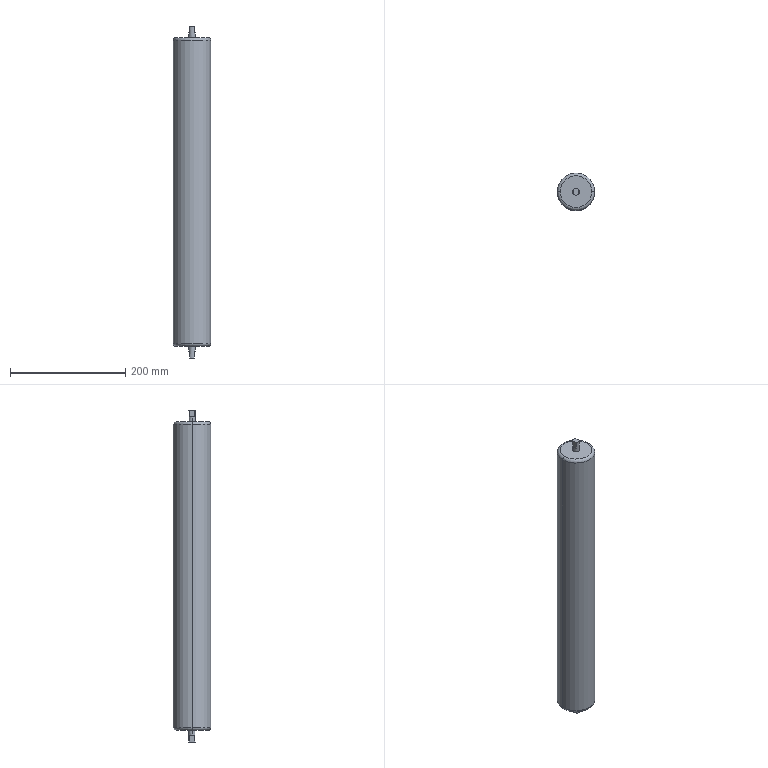Part | SolidWorks | features ICE 2, Extrusion 1, Fillet 1, MirrorPattern 1 | 1 solid | 22 faces | box 65 x 65 x 575 mm | volume 1777108 mm3 | plane 12 | cylinder 6 | torus 4 | commonest cylinder face diameters 12 x4 65 x2
STEP:
#1=CARTESIAN_POINT('',(-27.5,0.,-267.5));
#2=VERTEX_POINT('',#1);
#3=CARTESIAN_POINT('',(27.5,0.,-267.5));
#4=VERTEX_POINT('',#3);
#5=CARTESIAN_POINT('',(0.,0.,-267.5));
#6=DIRECTION('',(0.,0.,-1.));
#7=DIRECTION('',(1.,0.,0.));
#8=AXIS2_PLACEMENT_3D('',#5,#6,#7);
#9=CIRCLE('',#8,27.5);
#10=EDGE_CURVE('',#2,#4,#9,.T.);
#11=ORIENTED_EDGE('',*,*,#10,.F.);
#12=CARTESIAN_POINT('',(-32.5,0.,-262.5));
#13=VERTEX_POINT('',#12);
#14=CARTESIAN_POINT('',(-27.5,0.,-262.5));
#15=DIRECTION('',(0.,1.,0.));
#16=DIRECTION('',(-1.,0.,0.));
#17=AXIS2_PLACEMENT_3D('',#14,#15,#16);
#18=CIRCLE('',#17,5.);
#19=EDGE_CURVE('',#2,#13,#18,.T.);
#20=ORIENTED_EDGE('',*,*,#19,.T.);
#21=CARTESIAN_POINT('',(32.5,0.,-262.5));
#22=VERTEX_POINT('',#21);
#23=CARTESIAN_POINT('',(0.,0.,-262.5));
#24=DIRECTION('',(0.,0.,1.));
#25=DIRECTION('',(1.,0.,0.));
#26=AXIS2_PLACEMENT_3D('',#23,#24,#25);
#27=CIRCLE('',#26,32.5);
#28=EDGE_CURVE('',#22,#13,#27,.T.);
#29=ORIENTED_EDGE('',*,*,#28,.F.);
#30=CARTESIAN_POINT('',(27.5,0.,-262.5));
#31=DIRECTION('',(0.,-1.,0.));
#32=DIRECTION('',(0.,0.,-1.));
#33=AXIS2_PLACEMENT_3D('',#30,#31,#32);
#34=CIRCLE('',#33,5.);
#35=EDGE_CURVE('',#4,#22,#34,.T.);
#36=ORIENTED_EDGE('',*,*,#35,.F.);
#37=EDGE_LOOP('',(#11,#20,#29,#36));
#38=FACE_OUTER_BOUND('',#37,.T.);
#39=CARTESIAN_POINT('',(0.,0.,-262.5));
#40=DIRECTION('',(0.,0.,1.));
#41=DIRECTION('',(1.,0.,0.));
#42=AXIS2_PLACEMENT_3D('',#39,#40,#41);
#43=TOROIDAL_SURFACE('',#42,27.5,5.);
#44=ADVANCED_FACE('',(#38),#43,.T.);
#45=CARTESIAN_POINT('',(-32.5,0.,262.5));
#46=VERTEX_POINT('',#45);
#47=CARTESIAN_POINT('',(32.5,0.,262.5));
#48=VERTEX_POINT('',#47);
#49=CARTESIAN_POINT('',(0.,0.,262.5));
#50=DIRECTION('',(0.,0.,-1.));
#51=DIRECTION('',(1.,0.,0.));
#52=AXIS2_PLACEMENT_3D('',#49,#50,#51);
#53=CIRCLE('',#52,32.5);
#54=EDGE_CURVE('',#46,#48,#53,.T.);
#55=ORIENTED_EDGE('',*,*,#54,.F.);
#56=CARTESIAN_POINT('',(-27.5,0.,267.5));
#57=VERTEX_POINT('',#56);
#58=CARTESIAN_POINT('',(-27.5,0.,262.5));
#59=DIRECTION('',(0.,1.,0.));
#60=DIRECTION('',(-1.,0.,0.));
#61=AXIS2_PLACEMENT_3D('',#58,#59,#60);
#62=CIRCLE('',#61,5.);
#63=EDGE_CURVE('',#46,#57,#62,.T.);
#64=ORIENTED_EDGE('',*,*,#63,.T.);
#65=CARTESIAN_POINT('',(27.5,0.,267.5));
#66=VERTEX_POINT('',#65);
#67=CARTESIAN_POINT('',(0.,0.,267.5));
#68=DIRECTION('',(0.,0.,1.));
#69=DIRECTION('',(1.,0.,0.));
#70=AXIS2_PLACEMENT_3D('',#67,#68,#69);
#71=CIRCLE('',#70,27.5);
#72=EDGE_CURVE('',#66,#57,#71,.T.);
#73=ORIENTED_EDGE('',*,*,#72,.F.);
#74=CARTESIAN_POINT('',(27.5,0.,262.5));
#75=DIRECTION('',(0.,-1.,0.));
#76=DIRECTION('',(0.,0.,-1.));
#77=AXIS2_PLACEMENT_3D('',#74,#75,#76);
#78=CIRCLE('',#77,5.);
#79=EDGE_CURVE('',#48,#66,#78,.T.);
#80=ORIENTED_EDGE('',*,*,#79,.F.);
#81=EDGE_LOOP('',(#55,#64,#73,#80));
#82=FACE_OUTER_BOUND('',#81,.T.);
#83=CARTESIAN_POINT('',(0.,0.,262.5));
#84=DIRECTION('',(0.,0.,1.));
#85=DIRECTION('',(1.,0.,0.));
#86=AXIS2_PLACEMENT_3D('',#83,#84,#85);
#87=TOROIDAL_SURFACE('',#86,27.5,5.);
#88=ADVANCED_FACE('',(#82),#87,.T.);
#89=CARTESIAN_POINT('',(4.,4.472,275.5));
#90=VERTEX_POINT('',#89);
#91=CARTESIAN_POINT('',(6.,0.,275.5));
#92=VERTEX_POINT('',#91);
#93=CARTESIAN_POINT('',(0.,0.,275.5));
#94=DIRECTION('',(0.,0.,-1.));
#95=DIRECTION('',(1.,0.,0.));
#96=AXIS2_PLACEMENT_3D('',#93,#94,#95);
#97=CIRCLE('',#96,6.);
#98=EDGE_CURVE('',#90,#92,#97,.T.);
#99=ORIENTED_EDGE('',*,*,#98,.T.);
#100=CARTESIAN_POINT('',(6.,0.,267.5));
#101=VERTEX_POINT('',#100);
#102=CARTESIAN_POINT('',(6.,0.,287.5));
#103=DIRECTION('',(0.,0.,-1.));
#104=VECTOR('',#103,1000.);
#105=LINE('',#102,#104);
#106=EDGE_CURVE('',#92,#101,#105,.T.);
#107=ORIENTED_EDGE('',*,*,#106,.T.);
#108=CARTESIAN_POINT('',(-6.,0.,267.5));
#109=VERTEX_POINT('',#108);
#110=CARTESIAN_POINT('',(0.,0.,267.5));
#111=DIRECTION('',(0.,0.,1.));
#112=DIRECTION('',(1.,0.,0.));
#113=AXIS2_PLACEMENT_3D('',#110,#111,#112);
#114=CIRCLE('',#113,6.);
#115=EDGE_CURVE('',#101,#109,#114,.T.);
#116=ORIENTED_EDGE('',*,*,#115,.T.);
#117=CARTESIAN_POINT('',(-6.,0.,275.5));
#118=VERTEX_POINT('',#117);
#119=CARTESIAN_POINT('',(-6.,0.,287.5));
#120=DIRECTION('',(0.,0.,-1.));
#121=VECTOR('',#120,1000.);
#122=LINE('',#119,#121);
#123=EDGE_CURVE('',#118,#109,#122,.T.);
#124=ORIENTED_EDGE('',*,*,#123,.F.);
#125=CARTESIAN_POINT('',(-4.,4.472,275.5));
#126=VERTEX_POINT('',#125);
#127=CARTESIAN_POINT('',(0.,0.,275.5));
#128=DIRECTION('',(0.,0.,-1.));
#129=DIRECTION('',(1.,0.,0.));
#130=AXIS2_PLACEMENT_3D('',#127,#128,#129);
#131=CIRCLE('',#130,6.);
#132=EDGE_CURVE('',#118,#126,#131,.T.);
#133=ORIENTED_EDGE('',*,*,#132,.T.);
#134=CARTESIAN_POINT('',(-4.,4.472,287.5));
#135=VERTEX_POINT('',#134);
#136=CARTESIAN_POINT('',(-4.,4.472,287.5));
#137=DIRECTION('',(0.,0.,-1.));
#138=VECTOR('',#137,1000.);
#139=LINE('',#136,#138);
#140=EDGE_CURVE('',#135,#126,#139,.T.);
#141=ORIENTED_EDGE('',*,*,#140,.F.);
#142=CARTESIAN_POINT('',(4.,4.472,287.5));
#143=VERTEX_POINT('',#142);
#144=CARTESIAN_POINT('',(0.,0.,287.5));
#145=DIRECTION('',(0.,0.,-1.));
#146=DIRECTION('',(-1.,0.,0.));
#147=AXIS2_PLACEMENT_3D('',#144,#145,#146);
#148=CIRCLE('',#147,6.);
#149=EDGE_CURVE('',#135,#143,#148,.T.);
#150=ORIENTED_EDGE('',*,*,#149,.T.);
#151=CARTESIAN_POINT('',(4.,4.472,287.5));
#152=DIRECTION('',(0.,0.,1.));
#153=VECTOR('',#152,1000.);
#154=LINE('',#151,#153);
#155=EDGE_CURVE('',#90,#143,#154,.T.);
#156=ORIENTED_EDGE('',*,*,#155,.F.);
#157=EDGE_LOOP('',(#99,#107,#116,#124,#133,#141,#150,#156));
#158=FACE_OUTER_BOUND('',#157,.T.);
#159=CARTESIAN_POINT('',(0.,0.,287.5));
#160=DIRECTION('',(0.,0.,-1.));
#161=DIRECTION('',(-1.,0.,0.));
#162=AXIS2_PLACEMENT_3D('',#159,#160,#161);
#163=CYLINDRICAL_SURFACE('',#162,6.);
#164=ADVANCED_FACE('',(#158),#163,.T.);
#165=ORIENTED_EDGE('',*,*,#54,.T.);
#166=CARTESIAN_POINT('',(32.5,0.,267.5));
#167=DIRECTION('',(0.,0.,-1.));
#168=VECTOR('',#167,1000.);
#169=LINE('',#166,#168);
#170=EDGE_CURVE('',#48,#22,#169,.T.);
#171=ORIENTED_EDGE('',*,*,#170,.T.);
#172=ORIENTED_EDGE('',*,*,#28,.T.);
#173=CARTESIAN_POINT('',(-32.5,0.,267.5));
#174=DIRECTION('',(0.,0.,-1.));
#175=VECTOR('',#174,1000.);
#176=LINE('',#173,#175);
#177=EDGE_CURVE('',#46,#13,#176,.T.);
#178=ORIENTED_EDGE('',*,*,#177,.F.);
#179=EDGE_LOOP('',(#165,#171,#172,#178));
#180=FACE_OUTER_BOUND('',#179,.T.);
#181=CARTESIAN_POINT('',(0.,0.,267.5));
#182=DIRECTION('',(0.,0.,-1.));
#183=DIRECTION('',(-1.,0.,0.));
#184=AXIS2_PLACEMENT_3D('',#181,#182,#183);
#185=CYLINDRICAL_SURFACE('',#184,32.5);
#186=ADVANCED_FACE('',(#180),#185,.T.);
#187=CARTESIAN_POINT('',(-6.,0.,-275.5));
#188=VERTEX_POINT('',#187);
#189=CARTESIAN_POINT('',(-4.,4.472,-275.5));
#190=VERTEX_POINT('',#189);
#191=CARTESIAN_POINT('',(0.,0.,-275.5));
#192=DIRECTION('',(0.,0.,-1.));
#193=DIRECTION('',(-1.,0.,0.));
#194=AXIS2_PLACEMENT_3D('',#191,#192,#193);
#195=CIRCLE('',#194,6.);
#196=EDGE_CURVE('',#188,#190,#195,.T.);
#197=ORIENTED_EDGE('',*,*,#196,.F.);
#198=CARTESIAN_POINT('',(-6.,0.,-267.5));
#199=VERTEX_POINT('',#198);
#200=CARTESIAN_POINT('',(-6.,0.,-287.5));
#201=DIRECTION('',(0.,0.,1.));
#202=VECTOR('',#201,1000.);
#203=LINE('',#200,#202);
#204=EDGE_CURVE('',#188,#199,#203,.T.);
#205=ORIENTED_EDGE('',*,*,#204,.T.);
#206=CARTESIAN_POINT('',(6.,0.,-267.5));
#207=VERTEX_POINT('',#206);
#208=CARTESIAN_POINT('',(0.,0.,-267.5));
#209=DIRECTION('',(0.,0.,-1.));
#210=DIRECTION('',(1.,0.,0.));
#211=AXIS2_PLACEMENT_3D('',#208,#209,#210);
#212=CIRCLE('',#211,6.);
#213=EDGE_CURVE('',#199,#207,#212,.T.);
#214=ORIENTED_EDGE('',*,*,#213,.T.);
#215=CARTESIAN_POINT('',(6.,0.,-275.5));
#216=VERTEX_POINT('',#215);
#217=CARTESIAN_POINT('',(6.,0.,-287.5));
#218=DIRECTION('',(0.,0.,1.));
#219=VECTOR('',#218,1000.);
#220=LINE('',#217,#219);
#221=EDGE_CURVE('',#216,#207,#220,.T.);
#222=ORIENTED_EDGE('',*,*,#221,.F.);
#223=CARTESIAN_POINT('',(4.,4.472,-275.5));
#224=VERTEX_POINT('',#223);
#225=CARTESIAN_POINT('',(0.,0.,-275.5));
#226=DIRECTION('',(0.,0.,-1.));
#227=DIRECTION('',(-1.,0.,0.));
#228=AXIS2_PLACEMENT_3D('',#225,#226,#227);
#229=CIRCLE('',#228,6.);
#230=EDGE_CURVE('',#224,#216,#229,.T.);
#231=ORIENTED_EDGE('',*,*,#230,.F.);
#232=CARTESIAN_POINT('',(4.,4.472,-287.5));
#233=VERTEX_POINT('',#232);
#234=CARTESIAN_POINT('',(4.,4.472,-287.5));
#235=DIRECTION('',(0.,0.,1.));
#236=VECTOR('',#235,1000.);
#237=LINE('',#234,#236);
#238=EDGE_CURVE('',#233,#224,#237,.T.);
#239=ORIENTED_EDGE('',*,*,#238,.F.);
#240=CARTESIAN_POINT('',(-4.,4.472,-287.5));
#241=VERTEX_POINT('',#240);
#242=CARTESIAN_POINT('',(0.,0.,-287.5));
#243=DIRECTION('',(0.,0.,-1.));
#244=DIRECTION('',(-1.,0.,0.));
#245=AXIS2_PLACEMENT_3D('',#242,#243,#244);
#246=CIRCLE('',#245,6.);
#247=EDGE_CURVE('',#241,#233,#246,.T.);
#248=ORIENTED_EDGE('',*,*,#247,.F.);
#249=CARTESIAN_POINT('',(-4.,4.472,-287.5));
#250=DIRECTION('',(0.,0.,-1.));
#251=VECTOR('',#250,1000.);
#252=LINE('',#249,#251);
#253=EDGE_CURVE('',#190,#241,#252,.T.);
#254=ORIENTED_EDGE('',*,*,#253,.F.);
#255=EDGE_LOOP('',(#197,#205,#214,#222,#231,#239,#248,#254));
#256=FACE_OUTER_BOUND('',#255,.T.);
#257=CARTESIAN_POINT('',(0.,0.,-287.5));
#258=DIRECTION('',(0.,0.,1.));
#259=DIRECTION('',(1.,0.,0.));
#260=AXIS2_PLACEMENT_3D('',#257,#258,#259);
#261=CYLINDRICAL_SURFACE('',#260,6.);
#262=ADVANCED_FACE('',(#256),#261,.T.);
#263=ORIENTED_EDGE('',*,*,#204,.F.);
#264=CARTESIAN_POINT('',(-4.,-4.472,-275.5));
#265=VERTEX_POINT('',#264);
#266=CARTESIAN_POINT('',(0.,0.,-275.5));
#267=DIRECTION('',(0.,0.,-1.));
#268=DIRECTION('',(-1.,0.,0.));
#269=AXIS2_PLACEMENT_3D('',#266,#267,#268);
#270=CIRCLE('',#269,6.);
#271=EDGE_CURVE('',#265,#188,#270,.T.);
#272=ORIENTED_EDGE('',*,*,#271,.F.);
#273=CARTESIAN_POINT('',(-4.,-4.472,-287.5));
#274=VERTEX_POINT('',#273);
#275=CARTESIAN_POINT('',(-4.,-4.472,-287.5));
#276=DIRECTION('',(0.,0.,1.));
#277=VECTOR('',#276,1000.);
#278=LINE('',#275,#277);
#279=EDGE_CURVE('',#274,#265,#278,.T.);
#280=ORIENTED_EDGE('',*,*,#279,.F.);
#281=CARTESIAN_POINT('',(4.,-4.472,-287.5));
#282=VERTEX_POINT('',#281);
#283=CARTESIAN_POINT('',(0.,0.,-287.5));
#284=DIRECTION('',(0.,0.,-1.));
#285=DIRECTION('',(-1.,0.,0.));
#286=AXIS2_PLACEMENT_3D('',#283,#284,#285);
#287=CIRCLE('',#286,6.);
#288=EDGE_CURVE('',#282,#274,#287,.T.);
#289=ORIENTED_EDGE('',*,*,#288,.F.);
#290=CARTESIAN_POINT('',(4.,-4.472,-275.5));
#291=VERTEX_POINT('',#290);
#292=CARTESIAN_POINT('',(4.,-4.472,-287.5));
#293=DIRECTION('',(0.,0.,-1.));
#294=VECTOR('',#293,1000.);
#295=LINE('',#292,#294);
#296=EDGE_CURVE('',#291,#282,#295,.T.);
#297=ORIENTED_EDGE('',*,*,#296,.F.);
#298=CARTESIAN_POINT('',(0.,0.,-275.5));
#299=DIRECTION('',(0.,0.,-1.));
#300=DIRECTION('',(-1.,0.,0.));
#301=AXIS2_PLACEMENT_3D('',#298,#299,#300);
#302=CIRCLE('',#301,6.);
#303=EDGE_CURVE('',#216,#291,#302,.T.);
#304=ORIENTED_EDGE('',*,*,#303,.F.);
#305=ORIENTED_EDGE('',*,*,#221,.T.);
#306=CARTESIAN_POINT('',(0.,0.,-267.5));
#307=DIRECTION('',(0.,0.,-1.));
#308=DIRECTION('',(1.,0.,0.));
#309=AXIS2_PLACEMENT_3D('',#306,#307,#308);
#310=CIRCLE('',#309,6.);
#311=EDGE_CURVE('',#207,#199,#310,.T.);
#312=ORIENTED_EDGE('',*,*,#311,.T.);
#313=EDGE_LOOP('',(#263,#272,#280,#289,#297,#304,#305,#312));
#314=FACE_OUTER_BOUND('',#313,.T.);
#315=CARTESIAN_POINT('',(0.,0.,-287.5));
#316=DIRECTION('',(0.,0.,1.));
#317=DIRECTION('',(1.,0.,0.));
#318=AXIS2_PLACEMENT_3D('',#315,#316,#317);
#319=CYLINDRICAL_SURFACE('',#318,6.);
#320=ADVANCED_FACE('',(#314),#319,.T.);
#321=ORIENTED_EDGE('',*,*,#288,.T.);
#322=CARTESIAN_POINT('',(-4.,0.,-287.5));
#323=DIRECTION('',(0.,1.,0.));
#324=VECTOR('',#323,1000.);
#325=LINE('',#322,#324);
#326=EDGE_CURVE('',#274,#241,#325,.T.);
#327=ORIENTED_EDGE('',*,*,#326,.T.);
#328=ORIENTED_EDGE('',*,*,#247,.T.);
#329=CARTESIAN_POINT('',(4.,0.,-287.5));
#330=DIRECTION('',(0.,-1.,0.));
#331=VECTOR('',#330,1000.);
#332=LINE('',#329,#331);
#333=EDGE_CURVE('',#233,#282,#332,.T.);
#334=ORIENTED_EDGE('',*,*,#333,.T.);
#335=EDGE_LOOP('',(#321,#327,#328,#334));
#336=FACE_OUTER_BOUND('',#335,.T.);
#337=CARTESIAN_POINT('',(0.,0.,-287.5));
#338=DIRECTION('',(0.,0.,-1.));
#339=DIRECTION('',(-1.,0.,0.));
#340=AXIS2_PLACEMENT_3D('',#337,#338,#339);
#341=PLANE('',#340);
#342=ADVANCED_FACE('',(#336),#341,.T.);
#343=CARTESIAN_POINT('',(0.,0.,-267.5));
#344=DIRECTION('',(0.,0.,-1.));
#345=DIRECTION('',(1.,0.,0.));
#346=AXIS2_PLACEMENT_3D('',#343,#344,#345);
#347=CIRCLE('',#346,27.5);
#348=EDGE_CURVE('',#4,#2,#347,.T.);
#349=ORIENTED_EDGE('',*,*,#348,.T.);
#350=ORIENTED_EDGE('',*,*,#10,.T.);
#351=EDGE_LOOP('',(#349,#350));
#352=FACE_OUTER_BOUND('',#351,.T.);
#353=ORIENTED_EDGE('',*,*,#311,.F.);
#354=ORIENTED_EDGE('',*,*,#213,.F.);
#355=EDGE_LOOP('',(#353,#354));
#356=FACE_BOUND('',#355,.T.);
#357=CARTESIAN_POINT('',(0.,0.,-267.5));
#358=DIRECTION('',(0.,0.,1.));
#359=DIRECTION('',(1.,0.,0.));
#360=AXIS2_PLACEMENT_3D('',#357,#358,#359);
#361=PLANE('',#360);
#362=ADVANCED_FACE('',(#352,#356),#361,.F.);
#363=ORIENTED_EDGE('',*,*,#170,.F.);
#364=CARTESIAN_POINT('',(0.,0.,262.5));
#365=DIRECTION('',(0.,0.,-1.));
#366=DIRECTION('',(1.,0.,0.));
#367=AXIS2_PLACEMENT_3D('',#364,#365,#366);
#368=CIRCLE('',#367,32.5);
#369=EDGE_CURVE('',#48,#46,#368,.T.);
#370=ORIENTED_EDGE('',*,*,#369,.T.);
#371=ORIENTED_EDGE('',*,*,#177,.T.);
#372=CARTESIAN_POINT('',(0.,0.,-262.5));
#373=DIRECTION('',(0.,0.,1.));
#374=DIRECTION('',(1.,0.,0.));
#375=AXIS2_PLACEMENT_3D('',#372,#373,#374);
#376=CIRCLE('',#375,32.5);
#377=EDGE_CURVE('',#13,#22,#376,.T.);
#378=ORIENTED_EDGE('',*,*,#377,.T.);
#379=EDGE_LOOP('',(#363,#370,#371,#378));
#380=FACE_OUTER_BOUND('',#379,.T.);
#381=CARTESIAN_POINT('',(0.,0.,267.5));
#382=DIRECTION('',(0.,0.,-1.));
#383=DIRECTION('',(-1.,0.,0.));
#384=AXIS2_PLACEMENT_3D('',#381,#382,#383);
#385=CYLINDRICAL_SURFACE('',#384,32.5);
#386=ADVANCED_FACE('',(#380),#385,.T.);
#387=ORIENTED_EDGE('',*,*,#72,.T.);
#388=CARTESIAN_POINT('',(0.,0.,267.5));
#389=DIRECTION('',(0.,0.,1.));
#390=DIRECTION('',(1.,0.,0.));
#391=AXIS2_PLACEMENT_3D('',#388,#389,#390);
#392=CIRCLE('',#391,27.5);
#393=EDGE_CURVE('',#57,#66,#392,.T.);
#394=ORIENTED_EDGE('',*,*,#393,.T.);
#395=EDGE_LOOP('',(#387,#394));
#396=FACE_OUTER_BOUND('',#395,.T.);
#397=CARTESIAN_POINT('',(0.,0.,267.5));
#398=DIRECTION('',(0.,0.,1.));
#399=DIRECTION('',(1.,0.,0.));
#400=AXIS2_PLACEMENT_3D('',#397,#398,#399);
#401=CIRCLE('',#400,6.);
#402=EDGE_CURVE('',#109,#101,#401,.T.);
#403=ORIENTED_EDGE('',*,*,#402,.F.);
#404=ORIENTED_EDGE('',*,*,#115,.F.);
#405=EDGE_LOOP('',(#403,#404));
#406=FACE_BOUND('',#405,.T.);
#407=CARTESIAN_POINT('',(0.,0.,267.5));
#408=DIRECTION('',(0.,0.,1.));
#409=DIRECTION('',(1.,0.,0.));
#410=AXIS2_PLACEMENT_3D('',#407,#408,#409);
#411=PLANE('',#410);
#412=ADVANCED_FACE('',(#396,#406),#411,.T.);
#413=ORIENTED_EDGE('',*,*,#238,.T.);
#414=CARTESIAN_POINT('',(4.,6.421,-275.5));
#415=DIRECTION('',(0.,-1.,0.));
#416=VECTOR('',#415,1000.);
#417=LINE('',#414,#416);
#418=EDGE_CURVE('',#224,#291,#417,.T.);
#419=ORIENTED_EDGE('',*,*,#418,.T.);
#420=ORIENTED_EDGE('',*,*,#296,.T.);
#421=ORIENTED_EDGE('',*,*,#333,.F.);
#422=EDGE_LOOP('',(#413,#419,#420,#421));
#423=FACE_OUTER_BOUND('',#422,.T.);
#424=CARTESIAN_POINT('',(4.,6.421,-275.5));
#425=DIRECTION('',(1.,0.,0.));
#426=DIRECTION('',(0.,1.,0.));
#427=AXIS2_PLACEMENT_3D('',#424,#425,#426);
#428=PLANE('',#427);
#429=ADVANCED_FACE('',(#423),#428,.T.);
#430=ORIENTED_EDGE('',*,*,#230,.T.);
#431=ORIENTED_EDGE('',*,*,#303,.T.);
#432=ORIENTED_EDGE('',*,*,#418,.F.);
#433=EDGE_LOOP('',(#430,#431,#432));
#434=FACE_OUTER_BOUND('',#433,.T.);
#435=CARTESIAN_POINT('',(0.,0.,-275.5));
#436=DIRECTION('',(0.,0.,-1.));
#437=DIRECTION('',(-1.,0.,0.));
#438=AXIS2_PLACEMENT_3D('',#435,#436,#437);
#439=PLANE('',#438);
#440=ADVANCED_FACE('',(#434),#439,.T.);
#441=ORIENTED_EDGE('',*,*,#271,.T.);
#442=ORIENTED_EDGE('',*,*,#196,.T.);
#443=CARTESIAN_POINT('',(-4.,6.421,-275.5));
#444=DIRECTION('',(0.,1.,0.));
#445=VECTOR('',#444,1000.);
#446=LINE('',#443,#445);
#447=EDGE_CURVE('',#265,#190,#446,.T.);
#448=ORIENTED_EDGE('',*,*,#447,.F.);
#449=EDGE_LOOP('',(#441,#442,#448));
#450=FACE_OUTER_BOUND('',#449,.T.);
#451=CARTESIAN_POINT('',(0.,0.,-275.5));
#452=DIRECTION('',(0.,0.,-1.));
#453=DIRECTION('',(-1.,0.,0.));
#454=AXIS2_PLACEMENT_3D('',#451,#452,#453);
#455=PLANE('',#454);
#456=ADVANCED_FACE('',(#450),#455,.T.);
#457=ORIENTED_EDGE('',*,*,#279,.T.);
#458=ORIENTED_EDGE('',*,*,#447,.T.);
#459=ORIENTED_EDGE('',*,*,#253,.T.);
#460=ORIENTED_EDGE('',*,*,#326,.F.);
#461=EDGE_LOOP('',(#457,#458,#459,#460));
#462=FACE_OUTER_BOUND('',#461,.T.);
#463=CARTESIAN_POINT('',(-4.,6.421,-275.5));
#464=DIRECTION('',(-1.,0.,0.));
#465=DIRECTION('',(0.,-1.,0.));
#466=AXIS2_PLACEMENT_3D('',#463,#464,#465);
#467=PLANE('',#466);
#468=ADVANCED_FACE('',(#462),#467,.T.);
#469=ORIENTED_EDGE('',*,*,#106,.F.);
#470=CARTESIAN_POINT('',(4.,-4.472,275.5));
#471=VERTEX_POINT('',#470);
#472=CARTESIAN_POINT('',(0.,0.,275.5));
#473=DIRECTION('',(0.,0.,-1.));
#474=DIRECTION('',(1.,0.,0.));
#475=AXIS2_PLACEMENT_3D('',#472,#473,#474);
#476=CIRCLE('',#475,6.);
#477=EDGE_CURVE('',#92,#471,#476,.T.);
#478=ORIENTED_EDGE('',*,*,#477,.T.);
#479=CARTESIAN_POINT('',(4.,-4.472,287.5));
#480=VERTEX_POINT('',#479);
#481=CARTESIAN_POINT('',(4.,-4.472,287.5));
#482=DIRECTION('',(0.,0.,-1.));
#483=VECTOR('',#482,1000.);
#484=LINE('',#481,#483);
#485=EDGE_CURVE('',#480,#471,#484,.T.);
#486=ORIENTED_EDGE('',*,*,#485,.F.);
#487=CARTESIAN_POINT('',(-4.,-4.472,287.5));
#488=VERTEX_POINT('',#487);
#489=CARTESIAN_POINT('',(0.,0.,287.5));
#490=DIRECTION('',(0.,0.,-1.));
#491=DIRECTION('',(-1.,0.,0.));
#492=AXIS2_PLACEMENT_3D('',#489,#490,#491);
#493=CIRCLE('',#492,6.);
#494=EDGE_CURVE('',#480,#488,#493,.T.);
#495=ORIENTED_EDGE('',*,*,#494,.T.);
#496=CARTESIAN_POINT('',(-4.,-4.472,275.5));
#497=VERTEX_POINT('',#496);
#498=CARTESIAN_POINT('',(-4.,-4.472,287.5));
#499=DIRECTION('',(0.,0.,1.));
#500=VECTOR('',#499,1000.);
#501=LINE('',#498,#500);
#502=EDGE_CURVE('',#497,#488,#501,.T.);
#503=ORIENTED_EDGE('',*,*,#502,.F.);
#504=CARTESIAN_POINT('',(0.,0.,275.5));
#505=DIRECTION('',(0.,0.,-1.));
#506=DIRECTION('',(1.,0.,0.));
#507=AXIS2_PLACEMENT_3D('',#504,#505,#506);
#508=CIRCLE('',#507,6.);
#509=EDGE_CURVE('',#497,#118,#508,.T.);
#510=ORIENTED_EDGE('',*,*,#509,.T.);
#511=ORIENTED_EDGE('',*,*,#123,.T.);
#512=ORIENTED_EDGE('',*,*,#402,.T.);
#513=EDGE_LOOP('',(#469,#478,#486,#495,#503,#510,#511,#512));
#514=FACE_OUTER_BOUND('',#513,.T.);
#515=CARTESIAN_POINT('',(0.,0.,287.5));
#516=DIRECTION('',(0.,0.,-1.));
#517=DIRECTION('',(-1.,0.,0.));
#518=AXIS2_PLACEMENT_3D('',#515,#516,#517);
#519=CYLINDRICAL_SURFACE('',#518,6.);
#520=ADVANCED_FACE('',(#514),#519,.T.);
#521=CARTESIAN_POINT('',(-4.,0.,287.5));
#522=DIRECTION('',(0.,1.,0.));
#523=VECTOR('',#522,1000.);
#524=LINE('',#521,#523);
#525=EDGE_CURVE('',#488,#135,#524,.T.);
#526=ORIENTED_EDGE('',*,*,#525,.F.);
#527=ORIENTED_EDGE('',*,*,#494,.F.);
#528=CARTESIAN_POINT('',(4.,0.,287.5));
#529=DIRECTION('',(0.,-1.,0.));
#530=VECTOR('',#529,1000.);
#531=LINE('',#528,#530);
#532=EDGE_CURVE('',#143,#480,#531,.T.);
#533=ORIENTED_EDGE('',*,*,#532,.F.);
#534=ORIENTED_EDGE('',*,*,#149,.F.);
#535=EDGE_LOOP('',(#526,#527,#533,#534));
#536=FACE_OUTER_BOUND('',#535,.T.);
#537=CARTESIAN_POINT('',(0.,0.,287.5));
#538=DIRECTION('',(0.,0.,1.));
#539=DIRECTION('',(-1.,0.,0.));
#540=AXIS2_PLACEMENT_3D('',#537,#538,#539);
#541=PLANE('',#540);
#542=ADVANCED_FACE('',(#536),#541,.T.);
#543=ORIENTED_EDGE('',*,*,#155,.T.);
#544=ORIENTED_EDGE('',*,*,#532,.T.);
#545=ORIENTED_EDGE('',*,*,#485,.T.);
#546=CARTESIAN_POINT('',(4.,6.421,275.5));
#547=DIRECTION('',(0.,-1.,0.));
#548=VECTOR('',#547,1000.);
#549=LINE('',#546,#548);
#550=EDGE_CURVE('',#90,#471,#549,.T.);
#551=ORIENTED_EDGE('',*,*,#550,.F.);
#552=EDGE_LOOP('',(#543,#544,#545,#551));
#553=FACE_OUTER_BOUND('',#552,.T.);
#554=CARTESIAN_POINT('',(4.,6.421,275.5));
#555=DIRECTION('',(-1.,0.,0.));
#556=DIRECTION('',(0.,-1.,0.));
#557=AXIS2_PLACEMENT_3D('',#554,#555,#556);
#558=PLANE('',#557);
#559=ADVANCED_FACE('',(#553),#558,.F.);
#560=ORIENTED_EDGE('',*,*,#550,.T.);
#561=ORIENTED_EDGE('',*,*,#477,.F.);
#562=ORIENTED_EDGE('',*,*,#98,.F.);
#563=EDGE_LOOP('',(#560,#561,#562));
#564=FACE_OUTER_BOUND('',#563,.T.);
#565=CARTESIAN_POINT('',(0.,0.,275.5));
#566=DIRECTION('',(0.,0.,1.));
#567=DIRECTION('',(1.,0.,0.));
#568=AXIS2_PLACEMENT_3D('',#565,#566,#567);
#569=PLANE('',#568);
#570=ADVANCED_FACE('',(#564),#569,.T.);
#571=CARTESIAN_POINT('',(-4.,6.421,275.5));
#572=DIRECTION('',(0.,1.,0.));
#573=VECTOR('',#572,1000.);
#574=LINE('',#571,#573);
#575=EDGE_CURVE('',#497,#126,#574,.T.);
#576=ORIENTED_EDGE('',*,*,#575,.T.);
#577=ORIENTED_EDGE('',*,*,#132,.F.);
#578=ORIENTED_EDGE('',*,*,#509,.F.);
#579=EDGE_LOOP('',(#576,#577,#578));
#580=FACE_OUTER_BOUND('',#579,.T.);
#581=CARTESIAN_POINT('',(0.,0.,275.5));
#582=DIRECTION('',(0.,0.,1.));
#583=DIRECTION('',(1.,0.,0.));
#584=AXIS2_PLACEMENT_3D('',#581,#582,#583);
#585=PLANE('',#584);
#586=ADVANCED_FACE('',(#580),#585,.T.);
#587=ORIENTED_EDGE('',*,*,#502,.T.);
#588=ORIENTED_EDGE('',*,*,#525,.T.);
#589=ORIENTED_EDGE('',*,*,#140,.T.);
#590=ORIENTED_EDGE('',*,*,#575,.F.);
#591=EDGE_LOOP('',(#587,#588,#589,#590));
#592=FACE_OUTER_BOUND('',#591,.T.);
#593=CARTESIAN_POINT('',(-4.,6.421,275.5));
#594=DIRECTION('',(1.,0.,0.));
#595=DIRECTION('',(0.,1.,0.));
#596=AXIS2_PLACEMENT_3D('',#593,#594,#595);
#597=PLANE('',#596);
#598=ADVANCED_FACE('',(#592),#597,.F.);
#599=ORIENTED_EDGE('',*,*,#63,.F.);
#600=ORIENTED_EDGE('',*,*,#369,.F.);
#601=ORIENTED_EDGE('',*,*,#79,.T.);
#602=ORIENTED_EDGE('',*,*,#393,.F.);
#603=EDGE_LOOP('',(#599,#600,#601,#602));
#604=FACE_OUTER_BOUND('',#603,.T.);
#605=CARTESIAN_POINT('',(0.,0.,262.5));
#606=DIRECTION('',(0.,0.,1.));
#607=DIRECTION('',(1.,0.,0.));
#608=AXIS2_PLACEMENT_3D('',#605,#606,#607);
#609=TOROIDAL_SURFACE('',#608,27.5,5.);
#610=ADVANCED_FACE('',(#604),#609,.T.);
#611=ORIENTED_EDGE('',*,*,#19,.F.);
#612=ORIENTED_EDGE('',*,*,#348,.F.);
#613=ORIENTED_EDGE('',*,*,#35,.T.);
#614=ORIENTED_EDGE('',*,*,#377,.F.);
#615=EDGE_LOOP('',(#611,#612,#613,#614));
#616=FACE_OUTER_BOUND('',#615,.T.);
#617=CARTESIAN_POINT('',(0.,0.,-262.5));
#618=DIRECTION('',(0.,0.,1.));
#619=DIRECTION('',(1.,0.,0.));
#620=AXIS2_PLACEMENT_3D('',#617,#618,#619);
#621=TOROIDAL_SURFACE('',#620,27.5,5.);
#622=ADVANCED_FACE('',(#616),#621,.T.);
#623=CLOSED_SHELL('',(#44,#88,#164,#186,#262,#320,#342,#362,#386,#412,#429,#440,#456,#468,#520,#542,#559,#570,#586,#598,#610,#622));
#624=MANIFOLD_SOLID_BREP('',#623);
#625=CARTESIAN_POINT('',(0.,0.,0.));
#626=DIRECTION('',(0.,0.,1.));
#627=DIRECTION('',(1.,0.,0.));
#628=AXIS2_PLACEMENT_3D('',#625,#626,#627);
#629=(LENGTH_UNIT()NAMED_UNIT(*)SI_UNIT(.MILLI.,.METRE.));
#630=UNCERTAINTY_MEASURE_WITH_UNIT(LENGTH_MEASURE(0.00001),#629,'','');
#631=(NAMED_UNIT(*)PLANE_ANGLE_UNIT()SI_UNIT($,.RADIAN.));
#632=(NAMED_UNIT(*)SI_UNIT($,.STERADIAN.)SOLID_ANGLE_UNIT());
#633=(GEOMETRIC_REPRESENTATION_CONTEXT(3)GLOBAL_UNCERTAINTY_ASSIGNED_CONTEXT((#630))GLOBAL_UNIT_ASSIGNED_CONTEXT((#629,#631,#632))REPRESENTATION_CONTEXT('',''));
#634=ADVANCED_BREP_SHAPE_REPRESENTATION('',(#624,#628),#633);